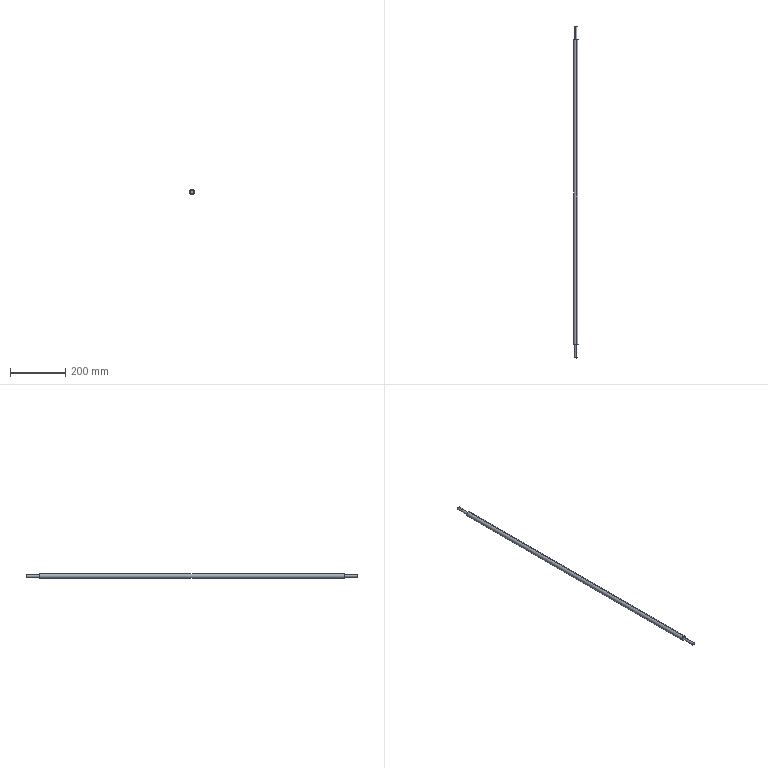Part | STEP file | Bevel gear fixed shaft | 1 solid | 10 faces | box 18 x 1200 x 18 mm | volume 287770 mm3 | cylinder 6 | plane 4 | commonest cylinder face diameters 10 x4 18 x2
STEP:
#1=CARTESIAN_POINT('',(0.,0.,0.));
#2=DIRECTION('',(0.,0.,1.));
#3=DIRECTION('',(1.,0.,0.));
#4=AXIS2_PLACEMENT_3D('',#1,#2,#3);
#5=CARTESIAN_POINT('',(-0.1276,1200.,4.929));
#6=VERTEX_POINT('',#5);
#7=CARTESIAN_POINT('',(-0.1276,1200.,-5.071));
#8=VERTEX_POINT('',#7);
#9=CARTESIAN_POINT('',(-0.1276,1200.,-0.07051));
#10=DIRECTION('',(0.,1.,0.));
#11=DIRECTION('',(0.,0.,1.));
#12=AXIS2_PLACEMENT_3D('',#9,#10,#11);
#13=CIRCLE('',#12,5.);
#14=CARTESIAN_POINT('',(-0.1276,1200.,-0.07051));
#15=DIRECTION('',(0.,-1.,0.));
#16=DIRECTION('',(0.,0.,-1.));
#17=AXIS2_PLACEMENT_3D('',#14,#15,#16);
#18=CYLINDRICAL_SURFACE('',#17,5.);
#19=CARTESIAN_POINT('',(3.142,0.));
#20=DIRECTION('',(-1.,0.));
#21=VECTOR('',#20,1.);
#22=LINE('',#19,#21);
#23=(GEOMETRIC_REPRESENTATION_CONTEXT(2)PARAMETRIC_REPRESENTATION_CONTEXT()REPRESENTATION_CONTEXT('',''));
#24=DEFINITIONAL_REPRESENTATION('',(#22),#23);
#25=PCURVE('',#18,#24);
#26=CARTESIAN_POINT('',(-0.1276,1200.,-0.07051));
#27=DIRECTION('',(0.,1.,0.));
#28=DIRECTION('',(0.,0.,1.));
#29=AXIS2_PLACEMENT_3D('',#26,#27,#28);
#30=PLANE('',#29);
#31=CARTESIAN_POINT('',(0.,0.));
#32=DIRECTION('',(1.,0.));
#33=AXIS2_PLACEMENT_2D('',#31,#32);
#34=CIRCLE('',#33,5.);
#35=(GEOMETRIC_REPRESENTATION_CONTEXT(2)PARAMETRIC_REPRESENTATION_CONTEXT()REPRESENTATION_CONTEXT('',''));
#36=DEFINITIONAL_REPRESENTATION('',(#34),#35);
#37=PCURVE('',#30,#36);
#38=SURFACE_CURVE('',#13,(#25,#37),.PCURVE_S1.);
#39=EDGE_CURVE('',#6,#8,#38,.T.);
#40=ORIENTED_EDGE('',*,*,#39,.F.);
#41=CARTESIAN_POINT('',(-0.1276,1150.,4.929));
#42=VERTEX_POINT('',#41);
#43=CARTESIAN_POINT('',(-0.1276,1200.,4.929));
#44=DIRECTION('',(0.,-1.,0.));
#45=VECTOR('',#44,1.);
#46=LINE('',#43,#45);
#47=CARTESIAN_POINT('',(3.142,0.));
#48=DIRECTION('',(0.,1.));
#49=VECTOR('',#48,1.);
#50=LINE('',#47,#49);
#51=(GEOMETRIC_REPRESENTATION_CONTEXT(2)PARAMETRIC_REPRESENTATION_CONTEXT()REPRESENTATION_CONTEXT('',''));
#52=DEFINITIONAL_REPRESENTATION('',(#50),#51);
#53=PCURVE('',#18,#52);
#54=CARTESIAN_POINT('',(-0.1276,1200.,-0.07051));
#55=DIRECTION('',(0.,-1.,0.));
#56=DIRECTION('',(0.,0.,-1.));
#57=AXIS2_PLACEMENT_3D('',#54,#55,#56);
#58=CYLINDRICAL_SURFACE('',#57,5.);
#59=CARTESIAN_POINT('',(3.142,0.));
#60=DIRECTION('',(0.,1.));
#61=VECTOR('',#60,1.);
#62=LINE('',#59,#61);
#63=(GEOMETRIC_REPRESENTATION_CONTEXT(2)PARAMETRIC_REPRESENTATION_CONTEXT()REPRESENTATION_CONTEXT('',''));
#64=DEFINITIONAL_REPRESENTATION('',(#62),#63);
#65=PCURVE('',#58,#64);
#66=SURFACE_CURVE('',#46,(#53,#65),.PCURVE_S1.);
#67=EDGE_CURVE('',#6,#42,#66,.T.);
#68=ORIENTED_EDGE('',*,*,#67,.T.);
#69=CARTESIAN_POINT('',(-0.1276,1150.,-5.071));
#70=VERTEX_POINT('',#69);
#71=CARTESIAN_POINT('',(-0.1276,1150.,-0.07051));
#72=DIRECTION('',(0.,1.,0.));
#73=DIRECTION('',(0.,0.,1.));
#74=AXIS2_PLACEMENT_3D('',#71,#72,#73);
#75=CIRCLE('',#74,5.);
#76=CARTESIAN_POINT('',(3.142,50.));
#77=DIRECTION('',(-1.,0.));
#78=VECTOR('',#77,1.);
#79=LINE('',#76,#78);
#80=(GEOMETRIC_REPRESENTATION_CONTEXT(2)PARAMETRIC_REPRESENTATION_CONTEXT()REPRESENTATION_CONTEXT('',''));
#81=DEFINITIONAL_REPRESENTATION('',(#79),#80);
#82=PCURVE('',#18,#81);
#83=CARTESIAN_POINT('',(0.,1150.,0.));
#84=DIRECTION('',(0.,1.,0.));
#85=DIRECTION('',(0.,0.,1.));
#86=AXIS2_PLACEMENT_3D('',#83,#84,#85);
#87=PLANE('',#86);
#88=CARTESIAN_POINT('',(-0.07051,-0.1276));
#89=DIRECTION('',(1.,0.));
#90=AXIS2_PLACEMENT_2D('',#88,#89);
#91=CIRCLE('',#90,5.);
#92=(GEOMETRIC_REPRESENTATION_CONTEXT(2)PARAMETRIC_REPRESENTATION_CONTEXT()REPRESENTATION_CONTEXT('',''));
#93=DEFINITIONAL_REPRESENTATION('',(#91),#92);
#94=PCURVE('',#87,#93);
#95=SURFACE_CURVE('',#75,(#82,#94),.PCURVE_S1.);
#96=EDGE_CURVE('',#42,#70,#95,.T.);
#97=ORIENTED_EDGE('',*,*,#96,.T.);
#98=CARTESIAN_POINT('',(-0.1276,1200.,-5.071));
#99=DIRECTION('',(0.,-1.,0.));
#100=VECTOR('',#99,1.);
#101=LINE('',#98,#100);
#102=CARTESIAN_POINT('',(0.,0.));
#103=DIRECTION('',(0.,1.));
#104=VECTOR('',#103,1.);
#105=LINE('',#102,#104);
#106=(GEOMETRIC_REPRESENTATION_CONTEXT(2)PARAMETRIC_REPRESENTATION_CONTEXT()REPRESENTATION_CONTEXT('',''));
#107=DEFINITIONAL_REPRESENTATION('',(#105),#106);
#108=PCURVE('',#18,#107);
#109=CARTESIAN_POINT('',(6.283,0.));
#110=DIRECTION('',(0.,1.));
#111=VECTOR('',#110,1.);
#112=LINE('',#109,#111);
#113=(GEOMETRIC_REPRESENTATION_CONTEXT(2)PARAMETRIC_REPRESENTATION_CONTEXT()REPRESENTATION_CONTEXT('',''));
#114=DEFINITIONAL_REPRESENTATION('',(#112),#113);
#115=PCURVE('',#58,#114);
#116=SURFACE_CURVE('',#101,(#108,#115),.PCURVE_S1.);
#117=EDGE_CURVE('',#8,#70,#116,.T.);
#118=ORIENTED_EDGE('',*,*,#117,.F.);
#119=EDGE_LOOP('',(#40,#68,#97,#118));
#120=FACE_BOUND('',#119,.T.);
#121=ADVANCED_FACE('',(#120),#18,.T.);
#122=CARTESIAN_POINT('',(0.,1150.,9.));
#123=VERTEX_POINT('',#122);
#124=CARTESIAN_POINT('',(0.,1150.,-9.));
#125=VERTEX_POINT('',#124);
#126=CARTESIAN_POINT('',(0.,1150.,0.));
#127=DIRECTION('',(0.,1.,0.));
#128=DIRECTION('',(0.,0.,1.));
#129=AXIS2_PLACEMENT_3D('',#126,#127,#128);
#130=CIRCLE('',#129,9.);
#131=CARTESIAN_POINT('',(0.,1150.,0.));
#132=DIRECTION('',(0.,-1.,0.));
#133=DIRECTION('',(0.,0.,-1.));
#134=AXIS2_PLACEMENT_3D('',#131,#132,#133);
#135=CYLINDRICAL_SURFACE('',#134,9.);
#136=CARTESIAN_POINT('',(3.142,0.));
#137=DIRECTION('',(-1.,0.));
#138=VECTOR('',#137,1.);
#139=LINE('',#136,#138);
#140=(GEOMETRIC_REPRESENTATION_CONTEXT(2)PARAMETRIC_REPRESENTATION_CONTEXT()REPRESENTATION_CONTEXT('',''));
#141=DEFINITIONAL_REPRESENTATION('',(#139),#140);
#142=PCURVE('',#135,#141);
#143=CARTESIAN_POINT('',(0.,0.));
#144=DIRECTION('',(1.,0.));
#145=AXIS2_PLACEMENT_2D('',#143,#144);
#146=CIRCLE('',#145,9.);
#147=(GEOMETRIC_REPRESENTATION_CONTEXT(2)PARAMETRIC_REPRESENTATION_CONTEXT()REPRESENTATION_CONTEXT('',''));
#148=DEFINITIONAL_REPRESENTATION('',(#146),#147);
#149=PCURVE('',#87,#148);
#150=SURFACE_CURVE('',#130,(#142,#149),.PCURVE_S1.);
#151=EDGE_CURVE('',#123,#125,#150,.T.);
#152=ORIENTED_EDGE('',*,*,#151,.F.);
#153=CARTESIAN_POINT('',(0.,50.,9.));
#154=VERTEX_POINT('',#153);
#155=CARTESIAN_POINT('',(0.,1150.,9.));
#156=DIRECTION('',(0.,-1.,0.));
#157=VECTOR('',#156,1.);
#158=LINE('',#155,#157);
#159=CARTESIAN_POINT('',(3.142,0.));
#160=DIRECTION('',(0.,1.));
#161=VECTOR('',#160,1.);
#162=LINE('',#159,#161);
#163=(GEOMETRIC_REPRESENTATION_CONTEXT(2)PARAMETRIC_REPRESENTATION_CONTEXT()REPRESENTATION_CONTEXT('',''));
#164=DEFINITIONAL_REPRESENTATION('',(#162),#163);
#165=PCURVE('',#135,#164);
#166=CARTESIAN_POINT('',(0.,1150.,0.));
#167=DIRECTION('',(0.,-1.,0.));
#168=DIRECTION('',(0.,0.,-1.));
#169=AXIS2_PLACEMENT_3D('',#166,#167,#168);
#170=CYLINDRICAL_SURFACE('',#169,9.);
#171=CARTESIAN_POINT('',(3.142,0.));
#172=DIRECTION('',(0.,1.));
#173=VECTOR('',#172,1.);
#174=LINE('',#171,#173);
#175=(GEOMETRIC_REPRESENTATION_CONTEXT(2)PARAMETRIC_REPRESENTATION_CONTEXT()REPRESENTATION_CONTEXT('',''));
#176=DEFINITIONAL_REPRESENTATION('',(#174),#175);
#177=PCURVE('',#170,#176);
#178=SURFACE_CURVE('',#158,(#165,#177),.PCURVE_S1.);
#179=EDGE_CURVE('',#123,#154,#178,.T.);
#180=ORIENTED_EDGE('',*,*,#179,.T.);
#181=CARTESIAN_POINT('',(0.,50.,-9.));
#182=VERTEX_POINT('',#181);
#183=CARTESIAN_POINT('',(0.,50.,0.));
#184=DIRECTION('',(0.,1.,0.));
#185=DIRECTION('',(0.,0.,1.));
#186=AXIS2_PLACEMENT_3D('',#183,#184,#185);
#187=CIRCLE('',#186,9.);
#188=CARTESIAN_POINT('',(3.142,1100.));
#189=DIRECTION('',(-1.,0.));
#190=VECTOR('',#189,1.);
#191=LINE('',#188,#190);
#192=(GEOMETRIC_REPRESENTATION_CONTEXT(2)PARAMETRIC_REPRESENTATION_CONTEXT()REPRESENTATION_CONTEXT('',''));
#193=DEFINITIONAL_REPRESENTATION('',(#191),#192);
#194=PCURVE('',#135,#193);
#195=CARTESIAN_POINT('',(0.,50.,0.));
#196=DIRECTION('',(0.,1.,0.));
#197=DIRECTION('',(0.,0.,1.));
#198=AXIS2_PLACEMENT_3D('',#195,#196,#197);
#199=PLANE('',#198);
#200=CARTESIAN_POINT('',(0.,0.));
#201=DIRECTION('',(1.,0.));
#202=AXIS2_PLACEMENT_2D('',#200,#201);
#203=CIRCLE('',#202,9.);
#204=(GEOMETRIC_REPRESENTATION_CONTEXT(2)PARAMETRIC_REPRESENTATION_CONTEXT()REPRESENTATION_CONTEXT('',''));
#205=DEFINITIONAL_REPRESENTATION('',(#203),#204);
#206=PCURVE('',#199,#205);
#207=SURFACE_CURVE('',#187,(#194,#206),.PCURVE_S1.);
#208=EDGE_CURVE('',#154,#182,#207,.T.);
#209=ORIENTED_EDGE('',*,*,#208,.T.);
#210=CARTESIAN_POINT('',(0.,1150.,-9.));
#211=DIRECTION('',(0.,-1.,0.));
#212=VECTOR('',#211,1.);
#213=LINE('',#210,#212);
#214=CARTESIAN_POINT('',(0.,0.));
#215=DIRECTION('',(0.,1.));
#216=VECTOR('',#215,1.);
#217=LINE('',#214,#216);
#218=(GEOMETRIC_REPRESENTATION_CONTEXT(2)PARAMETRIC_REPRESENTATION_CONTEXT()REPRESENTATION_CONTEXT('',''));
#219=DEFINITIONAL_REPRESENTATION('',(#217),#218);
#220=PCURVE('',#135,#219);
#221=CARTESIAN_POINT('',(6.283,0.));
#222=DIRECTION('',(0.,1.));
#223=VECTOR('',#222,1.);
#224=LINE('',#221,#223);
#225=(GEOMETRIC_REPRESENTATION_CONTEXT(2)PARAMETRIC_REPRESENTATION_CONTEXT()REPRESENTATION_CONTEXT('',''));
#226=DEFINITIONAL_REPRESENTATION('',(#224),#225);
#227=PCURVE('',#170,#226);
#228=SURFACE_CURVE('',#213,(#220,#227),.PCURVE_S1.);
#229=EDGE_CURVE('',#125,#182,#228,.T.);
#230=ORIENTED_EDGE('',*,*,#229,.F.);
#231=EDGE_LOOP('',(#152,#180,#209,#230));
#232=FACE_BOUND('',#231,.T.);
#233=ADVANCED_FACE('',(#232),#135,.T.);
#234=CARTESIAN_POINT('',(0.,50.,5.));
#235=VERTEX_POINT('',#234);
#236=CARTESIAN_POINT('',(0.,50.,-5.));
#237=VERTEX_POINT('',#236);
#238=CARTESIAN_POINT('',(0.,50.,0.));
#239=DIRECTION('',(0.,1.,0.));
#240=DIRECTION('',(0.,0.,1.));
#241=AXIS2_PLACEMENT_3D('',#238,#239,#240);
#242=CIRCLE('',#241,5.);
#243=CARTESIAN_POINT('',(0.,50.,0.));
#244=DIRECTION('',(0.,-1.,0.));
#245=DIRECTION('',(0.,0.,-1.));
#246=AXIS2_PLACEMENT_3D('',#243,#244,#245);
#247=CYLINDRICAL_SURFACE('',#246,5.);
#248=CARTESIAN_POINT('',(3.142,0.));
#249=DIRECTION('',(-1.,0.));
#250=VECTOR('',#249,1.);
#251=LINE('',#248,#250);
#252=(GEOMETRIC_REPRESENTATION_CONTEXT(2)PARAMETRIC_REPRESENTATION_CONTEXT()REPRESENTATION_CONTEXT('',''));
#253=DEFINITIONAL_REPRESENTATION('',(#251),#252);
#254=PCURVE('',#247,#253);
#255=CARTESIAN_POINT('',(0.,0.));
#256=DIRECTION('',(1.,0.));
#257=AXIS2_PLACEMENT_2D('',#255,#256);
#258=CIRCLE('',#257,5.);
#259=(GEOMETRIC_REPRESENTATION_CONTEXT(2)PARAMETRIC_REPRESENTATION_CONTEXT()REPRESENTATION_CONTEXT('',''));
#260=DEFINITIONAL_REPRESENTATION('',(#258),#259);
#261=PCURVE('',#199,#260);
#262=SURFACE_CURVE('',#242,(#254,#261),.PCURVE_S1.);
#263=EDGE_CURVE('',#235,#237,#262,.T.);
#264=ORIENTED_EDGE('',*,*,#263,.F.);
#265=CARTESIAN_POINT('',(0.,0.,5.));
#266=VERTEX_POINT('',#265);
#267=CARTESIAN_POINT('',(0.,50.,5.));
#268=DIRECTION('',(0.,-1.,0.));
#269=VECTOR('',#268,1.);
#270=LINE('',#267,#269);
#271=CARTESIAN_POINT('',(3.142,0.));
#272=DIRECTION('',(0.,1.));
#273=VECTOR('',#272,1.);
#274=LINE('',#271,#273);
#275=(GEOMETRIC_REPRESENTATION_CONTEXT(2)PARAMETRIC_REPRESENTATION_CONTEXT()REPRESENTATION_CONTEXT('',''));
#276=DEFINITIONAL_REPRESENTATION('',(#274),#275);
#277=PCURVE('',#247,#276);
#278=CARTESIAN_POINT('',(0.,50.,0.));
#279=DIRECTION('',(0.,-1.,0.));
#280=DIRECTION('',(0.,0.,-1.));
#281=AXIS2_PLACEMENT_3D('',#278,#279,#280);
#282=CYLINDRICAL_SURFACE('',#281,5.);
#283=CARTESIAN_POINT('',(3.142,0.));
#284=DIRECTION('',(0.,1.));
#285=VECTOR('',#284,1.);
#286=LINE('',#283,#285);
#287=(GEOMETRIC_REPRESENTATION_CONTEXT(2)PARAMETRIC_REPRESENTATION_CONTEXT()REPRESENTATION_CONTEXT('',''));
#288=DEFINITIONAL_REPRESENTATION('',(#286),#287);
#289=PCURVE('',#282,#288);
#290=SURFACE_CURVE('',#270,(#277,#289),.PCURVE_S1.);
#291=EDGE_CURVE('',#235,#266,#290,.T.);
#292=ORIENTED_EDGE('',*,*,#291,.T.);
#293=CARTESIAN_POINT('',(0.,0.,-5.));
#294=VERTEX_POINT('',#293);
#295=CARTESIAN_POINT('',(0.,0.,0.));
#296=DIRECTION('',(0.,1.,0.));
#297=DIRECTION('',(0.,0.,1.));
#298=AXIS2_PLACEMENT_3D('',#295,#296,#297);
#299=CIRCLE('',#298,5.);
#300=CARTESIAN_POINT('',(3.142,50.));
#301=DIRECTION('',(-1.,0.));
#302=VECTOR('',#301,1.);
#303=LINE('',#300,#302);
#304=(GEOMETRIC_REPRESENTATION_CONTEXT(2)PARAMETRIC_REPRESENTATION_CONTEXT()REPRESENTATION_CONTEXT('',''));
#305=DEFINITIONAL_REPRESENTATION('',(#303),#304);
#306=PCURVE('',#247,#305);
#307=CARTESIAN_POINT('',(0.,0.,0.));
#308=DIRECTION('',(0.,1.,0.));
#309=DIRECTION('',(0.,0.,1.));
#310=AXIS2_PLACEMENT_3D('',#307,#308,#309);
#311=PLANE('',#310);
#312=CARTESIAN_POINT('',(0.,0.));
#313=DIRECTION('',(1.,0.));
#314=AXIS2_PLACEMENT_2D('',#312,#313);
#315=CIRCLE('',#314,5.);
#316=(GEOMETRIC_REPRESENTATION_CONTEXT(2)PARAMETRIC_REPRESENTATION_CONTEXT()REPRESENTATION_CONTEXT('',''));
#317=DEFINITIONAL_REPRESENTATION('',(#315),#316);
#318=PCURVE('',#311,#317);
#319=SURFACE_CURVE('',#299,(#306,#318),.PCURVE_S1.);
#320=EDGE_CURVE('',#266,#294,#319,.T.);
#321=ORIENTED_EDGE('',*,*,#320,.T.);
#322=CARTESIAN_POINT('',(0.,50.,-5.));
#323=DIRECTION('',(0.,-1.,0.));
#324=VECTOR('',#323,1.);
#325=LINE('',#322,#324);
#326=CARTESIAN_POINT('',(0.,0.));
#327=DIRECTION('',(0.,1.));
#328=VECTOR('',#327,1.);
#329=LINE('',#326,#328);
#330=(GEOMETRIC_REPRESENTATION_CONTEXT(2)PARAMETRIC_REPRESENTATION_CONTEXT()REPRESENTATION_CONTEXT('',''));
#331=DEFINITIONAL_REPRESENTATION('',(#329),#330);
#332=PCURVE('',#247,#331);
#333=CARTESIAN_POINT('',(6.283,0.));
#334=DIRECTION('',(0.,1.));
#335=VECTOR('',#334,1.);
#336=LINE('',#333,#335);
#337=(GEOMETRIC_REPRESENTATION_CONTEXT(2)PARAMETRIC_REPRESENTATION_CONTEXT()REPRESENTATION_CONTEXT('',''));
#338=DEFINITIONAL_REPRESENTATION('',(#336),#337);
#339=PCURVE('',#282,#338);
#340=SURFACE_CURVE('',#325,(#332,#339),.PCURVE_S1.);
#341=EDGE_CURVE('',#237,#294,#340,.T.);
#342=ORIENTED_EDGE('',*,*,#341,.F.);
#343=EDGE_LOOP('',(#264,#292,#321,#342));
#344=FACE_BOUND('',#343,.T.);
#345=ADVANCED_FACE('',(#344),#247,.T.);
#346=ORIENTED_EDGE('',*,*,#291,.F.);
#347=CARTESIAN_POINT('',(0.,50.,0.));
#348=DIRECTION('',(0.,1.,0.));
#349=DIRECTION('',(0.,0.,1.));
#350=AXIS2_PLACEMENT_3D('',#347,#348,#349);
#351=CIRCLE('',#350,5.);
#352=CARTESIAN_POINT('',(9.425,0.));
#353=DIRECTION('',(-1.,0.));
#354=VECTOR('',#353,1.);
#355=LINE('',#352,#354);
#356=(GEOMETRIC_REPRESENTATION_CONTEXT(2)PARAMETRIC_REPRESENTATION_CONTEXT()REPRESENTATION_CONTEXT('',''));
#357=DEFINITIONAL_REPRESENTATION('',(#355),#356);
#358=PCURVE('',#282,#357);
#359=CARTESIAN_POINT('',(0.,0.));
#360=DIRECTION('',(1.,0.));
#361=AXIS2_PLACEMENT_2D('',#359,#360);
#362=CIRCLE('',#361,5.);
#363=(GEOMETRIC_REPRESENTATION_CONTEXT(2)PARAMETRIC_REPRESENTATION_CONTEXT()REPRESENTATION_CONTEXT('',''));
#364=DEFINITIONAL_REPRESENTATION('',(#362),#363);
#365=PCURVE('',#199,#364);
#366=SURFACE_CURVE('',#351,(#358,#365),.PCURVE_S1.);
#367=EDGE_CURVE('',#237,#235,#366,.T.);
#368=ORIENTED_EDGE('',*,*,#367,.F.);
#369=ORIENTED_EDGE('',*,*,#341,.T.);
#370=CARTESIAN_POINT('',(0.,0.,0.));
#371=DIRECTION('',(0.,1.,0.));
#372=DIRECTION('',(0.,0.,1.));
#373=AXIS2_PLACEMENT_3D('',#370,#371,#372);
#374=CIRCLE('',#373,5.);
#375=CARTESIAN_POINT('',(9.425,50.));
#376=DIRECTION('',(-1.,0.));
#377=VECTOR('',#376,1.);
#378=LINE('',#375,#377);
#379=(GEOMETRIC_REPRESENTATION_CONTEXT(2)PARAMETRIC_REPRESENTATION_CONTEXT()REPRESENTATION_CONTEXT('',''));
#380=DEFINITIONAL_REPRESENTATION('',(#378),#379);
#381=PCURVE('',#282,#380);
#382=CARTESIAN_POINT('',(0.,0.));
#383=DIRECTION('',(1.,0.));
#384=AXIS2_PLACEMENT_2D('',#382,#383);
#385=CIRCLE('',#384,5.);
#386=(GEOMETRIC_REPRESENTATION_CONTEXT(2)PARAMETRIC_REPRESENTATION_CONTEXT()REPRESENTATION_CONTEXT('',''));
#387=DEFINITIONAL_REPRESENTATION('',(#385),#386);
#388=PCURVE('',#311,#387);
#389=SURFACE_CURVE('',#374,(#381,#388),.PCURVE_S1.);
#390=EDGE_CURVE('',#294,#266,#389,.T.);
#391=ORIENTED_EDGE('',*,*,#390,.T.);
#392=EDGE_LOOP('',(#346,#368,#369,#391));
#393=FACE_BOUND('',#392,.T.);
#394=ADVANCED_FACE('',(#393),#282,.T.);
#395=ORIENTED_EDGE('',*,*,#390,.F.);
#396=ORIENTED_EDGE('',*,*,#320,.F.);
#397=EDGE_LOOP('',(#395,#396));
#398=FACE_BOUND('',#397,.T.);
#399=ADVANCED_FACE('',(#398),#311,.F.);
#400=CARTESIAN_POINT('',(0.,50.,0.));
#401=DIRECTION('',(0.,1.,0.));
#402=DIRECTION('',(0.,0.,1.));
#403=AXIS2_PLACEMENT_3D('',#400,#401,#402);
#404=CIRCLE('',#403,9.);
#405=CARTESIAN_POINT('',(0.,0.));
#406=DIRECTION('',(1.,0.));
#407=AXIS2_PLACEMENT_2D('',#405,#406);
#408=CIRCLE('',#407,9.);
#409=(GEOMETRIC_REPRESENTATION_CONTEXT(2)PARAMETRIC_REPRESENTATION_CONTEXT()REPRESENTATION_CONTEXT('',''));
#410=DEFINITIONAL_REPRESENTATION('',(#408),#409);
#411=PCURVE('',#199,#410);
#412=CARTESIAN_POINT('',(9.425,1100.));
#413=DIRECTION('',(-1.,0.));
#414=VECTOR('',#413,1.);
#415=LINE('',#412,#414);
#416=(GEOMETRIC_REPRESENTATION_CONTEXT(2)PARAMETRIC_REPRESENTATION_CONTEXT()REPRESENTATION_CONTEXT('',''));
#417=DEFINITIONAL_REPRESENTATION('',(#415),#416);
#418=PCURVE('',#170,#417);
#419=SURFACE_CURVE('',#404,(#411,#418),.PCURVE_S1.);
#420=EDGE_CURVE('',#182,#154,#419,.T.);
#421=ORIENTED_EDGE('',*,*,#420,.F.);
#422=ORIENTED_EDGE('',*,*,#208,.F.);
#423=EDGE_LOOP('',(#421,#422));
#424=FACE_BOUND('',#423,.T.);
#425=ORIENTED_EDGE('',*,*,#367,.T.);
#426=ORIENTED_EDGE('',*,*,#263,.T.);
#427=EDGE_LOOP('',(#425,#426));
#428=FACE_BOUND('',#427,.T.);
#429=ADVANCED_FACE('',(#424,#428),#199,.F.);
#430=ORIENTED_EDGE('',*,*,#179,.F.);
#431=CARTESIAN_POINT('',(0.,1150.,0.));
#432=DIRECTION('',(0.,1.,0.));
#433=DIRECTION('',(0.,0.,1.));
#434=AXIS2_PLACEMENT_3D('',#431,#432,#433);
#435=CIRCLE('',#434,9.);
#436=CARTESIAN_POINT('',(9.425,0.));
#437=DIRECTION('',(-1.,0.));
#438=VECTOR('',#437,1.);
#439=LINE('',#436,#438);
#440=(GEOMETRIC_REPRESENTATION_CONTEXT(2)PARAMETRIC_REPRESENTATION_CONTEXT()REPRESENTATION_CONTEXT('',''));
#441=DEFINITIONAL_REPRESENTATION('',(#439),#440);
#442=PCURVE('',#170,#441);
#443=CARTESIAN_POINT('',(0.,0.));
#444=DIRECTION('',(1.,0.));
#445=AXIS2_PLACEMENT_2D('',#443,#444);
#446=CIRCLE('',#445,9.);
#447=(GEOMETRIC_REPRESENTATION_CONTEXT(2)PARAMETRIC_REPRESENTATION_CONTEXT()REPRESENTATION_CONTEXT('',''));
#448=DEFINITIONAL_REPRESENTATION('',(#446),#447);
#449=PCURVE('',#87,#448);
#450=SURFACE_CURVE('',#435,(#442,#449),.PCURVE_S1.);
#451=EDGE_CURVE('',#125,#123,#450,.T.);
#452=ORIENTED_EDGE('',*,*,#451,.F.);
#453=ORIENTED_EDGE('',*,*,#229,.T.);
#454=ORIENTED_EDGE('',*,*,#420,.T.);
#455=EDGE_LOOP('',(#430,#452,#453,#454));
#456=FACE_BOUND('',#455,.T.);
#457=ADVANCED_FACE('',(#456),#170,.T.);
#458=CARTESIAN_POINT('',(-0.1276,1150.,-0.07051));
#459=DIRECTION('',(0.,1.,0.));
#460=DIRECTION('',(0.,0.,1.));
#461=AXIS2_PLACEMENT_3D('',#458,#459,#460);
#462=CIRCLE('',#461,5.);
#463=CARTESIAN_POINT('',(-0.07051,-0.1276));
#464=DIRECTION('',(1.,0.));
#465=AXIS2_PLACEMENT_2D('',#463,#464);
#466=CIRCLE('',#465,5.);
#467=(GEOMETRIC_REPRESENTATION_CONTEXT(2)PARAMETRIC_REPRESENTATION_CONTEXT()REPRESENTATION_CONTEXT('',''));
#468=DEFINITIONAL_REPRESENTATION('',(#466),#467);
#469=PCURVE('',#87,#468);
#470=CARTESIAN_POINT('',(9.425,50.));
#471=DIRECTION('',(-1.,0.));
#472=VECTOR('',#471,1.);
#473=LINE('',#470,#472);
#474=(GEOMETRIC_REPRESENTATION_CONTEXT(2)PARAMETRIC_REPRESENTATION_CONTEXT()REPRESENTATION_CONTEXT('',''));
#475=DEFINITIONAL_REPRESENTATION('',(#473),#474);
#476=PCURVE('',#58,#475);
#477=SURFACE_CURVE('',#462,(#469,#476),.PCURVE_S1.);
#478=EDGE_CURVE('',#70,#42,#477,.T.);
#479=ORIENTED_EDGE('',*,*,#478,.F.);
#480=ORIENTED_EDGE('',*,*,#96,.F.);
#481=EDGE_LOOP('',(#479,#480));
#482=FACE_BOUND('',#481,.T.);
#483=ORIENTED_EDGE('',*,*,#451,.T.);
#484=ORIENTED_EDGE('',*,*,#151,.T.);
#485=EDGE_LOOP('',(#483,#484));
#486=FACE_BOUND('',#485,.T.);
#487=ADVANCED_FACE('',(#482,#486),#87,.T.);
#488=ORIENTED_EDGE('',*,*,#67,.F.);
#489=CARTESIAN_POINT('',(-0.1276,1200.,-0.07051));
#490=DIRECTION('',(0.,1.,0.));
#491=DIRECTION('',(0.,0.,1.));
#492=AXIS2_PLACEMENT_3D('',#489,#490,#491);
#493=CIRCLE('',#492,5.);
#494=CARTESIAN_POINT('',(9.425,0.));
#495=DIRECTION('',(-1.,0.));
#496=VECTOR('',#495,1.);
#497=LINE('',#494,#496);
#498=(GEOMETRIC_REPRESENTATION_CONTEXT(2)PARAMETRIC_REPRESENTATION_CONTEXT()REPRESENTATION_CONTEXT('',''));
#499=DEFINITIONAL_REPRESENTATION('',(#497),#498);
#500=PCURVE('',#58,#499);
#501=CARTESIAN_POINT('',(0.,0.));
#502=DIRECTION('',(1.,0.));
#503=AXIS2_PLACEMENT_2D('',#501,#502);
#504=CIRCLE('',#503,5.);
#505=(GEOMETRIC_REPRESENTATION_CONTEXT(2)PARAMETRIC_REPRESENTATION_CONTEXT()REPRESENTATION_CONTEXT('',''));
#506=DEFINITIONAL_REPRESENTATION('',(#504),#505);
#507=PCURVE('',#30,#506);
#508=SURFACE_CURVE('',#493,(#500,#507),.PCURVE_S1.);
#509=EDGE_CURVE('',#8,#6,#508,.T.);
#510=ORIENTED_EDGE('',*,*,#509,.F.);
#511=ORIENTED_EDGE('',*,*,#117,.T.);
#512=ORIENTED_EDGE('',*,*,#478,.T.);
#513=EDGE_LOOP('',(#488,#510,#511,#512));
#514=FACE_BOUND('',#513,.T.);
#515=ADVANCED_FACE('',(#514),#58,.T.);
#516=ORIENTED_EDGE('',*,*,#509,.T.);
#517=ORIENTED_EDGE('',*,*,#39,.T.);
#518=EDGE_LOOP('',(#516,#517));
#519=FACE_BOUND('',#518,.T.);
#520=ADVANCED_FACE('',(#519),#30,.T.);
#521=CLOSED_SHELL('',(#121,#233,#345,#394,#399,#429,#457,#487,#515,#520));
#522=MANIFOLD_SOLID_BREP('',#521);
#523=(LENGTH_UNIT()NAMED_UNIT(*)SI_UNIT(.MILLI.,.METRE.));
#524=UNCERTAINTY_MEASURE_WITH_UNIT(LENGTH_MEASURE(0.0000001),#523,'','');
#525=(NAMED_UNIT(*)PLANE_ANGLE_UNIT()SI_UNIT($,.RADIAN.));
#526=(NAMED_UNIT(*)SI_UNIT($,.STERADIAN.)SOLID_ANGLE_UNIT());
#527=(GEOMETRIC_REPRESENTATION_CONTEXT(3)GLOBAL_UNCERTAINTY_ASSIGNED_CONTEXT((#524))GLOBAL_UNIT_ASSIGNED_CONTEXT((#523,#525,#526))REPRESENTATION_CONTEXT('',''));
#528=ADVANCED_BREP_SHAPE_REPRESENTATION('',(#4,#522),#527);